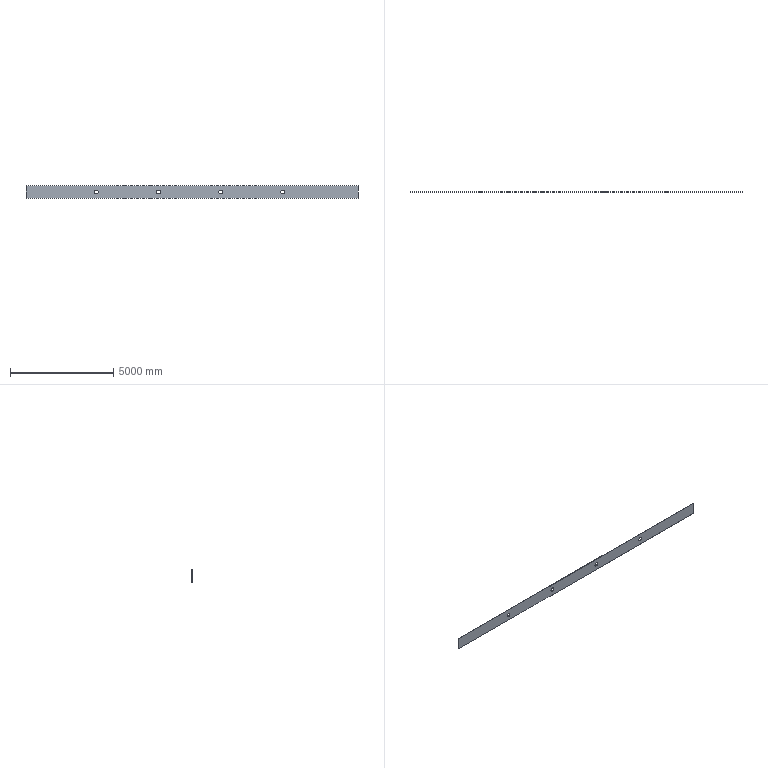Part | SolidWorks | features Cut 1, Extrusion 1, LPattern 1 | 1 solid | 14 faces | box 16040 x 12 x 600 mm | volume 114266549 mm3 | cylinder 8 | plane 6 | commonest cylinder face diameters 180 x8
STEP:
#1=CARTESIAN_POINT('',(-1620.,0.,-90.));
#2=VERTEX_POINT('',#1);
#3=CARTESIAN_POINT('',(-1620.,0.,90.));
#4=VERTEX_POINT('',#3);
#5=CARTESIAN_POINT('',(-1620.,0.,0.));
#6=DIRECTION('',(0.,1.,0.));
#7=DIRECTION('',(0.,0.,1.));
#8=AXIS2_PLACEMENT_3D('',#5,#6,#7);
#9=CIRCLE('',#8,90.);
#10=EDGE_CURVE('',#2,#4,#9,.T.);
#11=ORIENTED_EDGE('',*,*,#10,.F.);
#12=CARTESIAN_POINT('',(-1620.,12.,-90.));
#13=VERTEX_POINT('',#12);
#14=CARTESIAN_POINT('',(-1620.,0.,-90.));
#15=DIRECTION('',(0.,1.,0.));
#16=VECTOR('',#15,1000.);
#17=LINE('',#14,#16);
#18=EDGE_CURVE('',#2,#13,#17,.T.);
#19=ORIENTED_EDGE('',*,*,#18,.T.);
#20=CARTESIAN_POINT('',(-1620.,12.,90.));
#21=VERTEX_POINT('',#20);
#22=CARTESIAN_POINT('',(-1620.,12.,0.));
#23=DIRECTION('',(0.,1.,0.));
#24=DIRECTION('',(0.,0.,1.));
#25=AXIS2_PLACEMENT_3D('',#22,#23,#24);
#26=CIRCLE('',#25,90.);
#27=EDGE_CURVE('',#13,#21,#26,.T.);
#28=ORIENTED_EDGE('',*,*,#27,.T.);
#29=CARTESIAN_POINT('',(-1620.,0.,90.));
#30=DIRECTION('',(0.,1.,0.));
#31=VECTOR('',#30,1000.);
#32=LINE('',#29,#31);
#33=EDGE_CURVE('',#4,#21,#32,.T.);
#34=ORIENTED_EDGE('',*,*,#33,.F.);
#35=EDGE_LOOP('',(#11,#19,#28,#34));
#36=FACE_OUTER_BOUND('',#35,.T.);
#37=CARTESIAN_POINT('',(-1620.,0.,0.));
#38=DIRECTION('',(0.,1.,0.));
#39=DIRECTION('',(0.,0.,1.));
#40=AXIS2_PLACEMENT_3D('',#37,#38,#39);
#41=CYLINDRICAL_SURFACE('',#40,90.);
#42=ADVANCED_FACE('',(#36),#41,.F.);
#43=CARTESIAN_POINT('',(-4620.,0.,-90.));
#44=VERTEX_POINT('',#43);
#45=CARTESIAN_POINT('',(-4620.,0.,90.));
#46=VERTEX_POINT('',#45);
#47=CARTESIAN_POINT('',(-4620.,0.,0.));
#48=DIRECTION('',(0.,1.,0.));
#49=DIRECTION('',(0.,0.,1.));
#50=AXIS2_PLACEMENT_3D('',#47,#48,#49);
#51=CIRCLE('',#50,90.);
#52=EDGE_CURVE('',#44,#46,#51,.T.);
#53=ORIENTED_EDGE('',*,*,#52,.F.);
#54=CARTESIAN_POINT('',(-4620.,12.,-90.));
#55=VERTEX_POINT('',#54);
#56=CARTESIAN_POINT('',(-4620.,0.,-90.));
#57=DIRECTION('',(0.,1.,0.));
#58=VECTOR('',#57,1000.);
#59=LINE('',#56,#58);
#60=EDGE_CURVE('',#44,#55,#59,.T.);
#61=ORIENTED_EDGE('',*,*,#60,.T.);
#62=CARTESIAN_POINT('',(-4620.,12.,90.));
#63=VERTEX_POINT('',#62);
#64=CARTESIAN_POINT('',(-4620.,12.,0.));
#65=DIRECTION('',(0.,1.,0.));
#66=DIRECTION('',(0.,0.,1.));
#67=AXIS2_PLACEMENT_3D('',#64,#65,#66);
#68=CIRCLE('',#67,90.);
#69=EDGE_CURVE('',#55,#63,#68,.T.);
#70=ORIENTED_EDGE('',*,*,#69,.T.);
#71=CARTESIAN_POINT('',(-4620.,0.,90.));
#72=DIRECTION('',(0.,1.,0.));
#73=VECTOR('',#72,1000.);
#74=LINE('',#71,#73);
#75=EDGE_CURVE('',#46,#63,#74,.T.);
#76=ORIENTED_EDGE('',*,*,#75,.F.);
#77=EDGE_LOOP('',(#53,#61,#70,#76));
#78=FACE_OUTER_BOUND('',#77,.T.);
#79=CARTESIAN_POINT('',(-4620.,0.,0.));
#80=DIRECTION('',(0.,1.,0.));
#81=DIRECTION('',(0.,0.,1.));
#82=AXIS2_PLACEMENT_3D('',#79,#80,#81);
#83=CYLINDRICAL_SURFACE('',#82,90.);
#84=ADVANCED_FACE('',(#78),#83,.F.);
#85=CARTESIAN_POINT('',(1380.,0.,-90.));
#86=VERTEX_POINT('',#85);
#87=CARTESIAN_POINT('',(1380.,0.,90.));
#88=VERTEX_POINT('',#87);
#89=CARTESIAN_POINT('',(1380.,0.,0.));
#90=DIRECTION('',(0.,1.,0.));
#91=DIRECTION('',(0.,0.,1.));
#92=AXIS2_PLACEMENT_3D('',#89,#90,#91);
#93=CIRCLE('',#92,90.);
#94=EDGE_CURVE('',#86,#88,#93,.T.);
#95=ORIENTED_EDGE('',*,*,#94,.F.);
#96=CARTESIAN_POINT('',(1380.,12.,-90.));
#97=VERTEX_POINT('',#96);
#98=CARTESIAN_POINT('',(1380.,0.,-90.));
#99=DIRECTION('',(0.,1.,0.));
#100=VECTOR('',#99,1000.);
#101=LINE('',#98,#100);
#102=EDGE_CURVE('',#86,#97,#101,.T.);
#103=ORIENTED_EDGE('',*,*,#102,.T.);
#104=CARTESIAN_POINT('',(1380.,12.,90.));
#105=VERTEX_POINT('',#104);
#106=CARTESIAN_POINT('',(1380.,12.,0.));
#107=DIRECTION('',(0.,1.,0.));
#108=DIRECTION('',(0.,0.,1.));
#109=AXIS2_PLACEMENT_3D('',#106,#107,#108);
#110=CIRCLE('',#109,90.);
#111=EDGE_CURVE('',#97,#105,#110,.T.);
#112=ORIENTED_EDGE('',*,*,#111,.T.);
#113=CARTESIAN_POINT('',(1380.,0.,90.));
#114=DIRECTION('',(0.,1.,0.));
#115=VECTOR('',#114,1000.);
#116=LINE('',#113,#115);
#117=EDGE_CURVE('',#88,#105,#116,.T.);
#118=ORIENTED_EDGE('',*,*,#117,.F.);
#119=EDGE_LOOP('',(#95,#103,#112,#118));
#120=FACE_OUTER_BOUND('',#119,.T.);
#121=CARTESIAN_POINT('',(1380.,0.,0.));
#122=DIRECTION('',(0.,1.,0.));
#123=DIRECTION('',(0.,0.,1.));
#124=AXIS2_PLACEMENT_3D('',#121,#122,#123);
#125=CYLINDRICAL_SURFACE('',#124,90.);
#126=ADVANCED_FACE('',(#120),#125,.F.);
#127=CARTESIAN_POINT('',(4380.,0.,-90.));
#128=VERTEX_POINT('',#127);
#129=CARTESIAN_POINT('',(4380.,0.,90.));
#130=VERTEX_POINT('',#129);
#131=CARTESIAN_POINT('',(4380.,0.,0.));
#132=DIRECTION('',(0.,1.,0.));
#133=DIRECTION('',(0.,0.,1.));
#134=AXIS2_PLACEMENT_3D('',#131,#132,#133);
#135=CIRCLE('',#134,90.);
#136=EDGE_CURVE('',#128,#130,#135,.T.);
#137=ORIENTED_EDGE('',*,*,#136,.F.);
#138=CARTESIAN_POINT('',(4380.,12.,-90.));
#139=VERTEX_POINT('',#138);
#140=CARTESIAN_POINT('',(4380.,0.,-90.));
#141=DIRECTION('',(0.,1.,0.));
#142=VECTOR('',#141,1000.);
#143=LINE('',#140,#142);
#144=EDGE_CURVE('',#128,#139,#143,.T.);
#145=ORIENTED_EDGE('',*,*,#144,.T.);
#146=CARTESIAN_POINT('',(4380.,12.,90.));
#147=VERTEX_POINT('',#146);
#148=CARTESIAN_POINT('',(4380.,12.,0.));
#149=DIRECTION('',(0.,1.,0.));
#150=DIRECTION('',(0.,0.,1.));
#151=AXIS2_PLACEMENT_3D('',#148,#149,#150);
#152=CIRCLE('',#151,90.);
#153=EDGE_CURVE('',#139,#147,#152,.T.);
#154=ORIENTED_EDGE('',*,*,#153,.T.);
#155=CARTESIAN_POINT('',(4380.,0.,90.));
#156=DIRECTION('',(0.,1.,0.));
#157=VECTOR('',#156,1000.);
#158=LINE('',#155,#157);
#159=EDGE_CURVE('',#130,#147,#158,.T.);
#160=ORIENTED_EDGE('',*,*,#159,.F.);
#161=EDGE_LOOP('',(#137,#145,#154,#160));
#162=FACE_OUTER_BOUND('',#161,.T.);
#163=CARTESIAN_POINT('',(4380.,0.,0.));
#164=DIRECTION('',(0.,1.,0.));
#165=DIRECTION('',(0.,0.,1.));
#166=AXIS2_PLACEMENT_3D('',#163,#164,#165);
#167=CYLINDRICAL_SURFACE('',#166,90.);
#168=ADVANCED_FACE('',(#162),#167,.F.);
#169=ORIENTED_EDGE('',*,*,#144,.F.);
#170=CARTESIAN_POINT('',(4380.,0.,0.));
#171=DIRECTION('',(0.,1.,0.));
#172=DIRECTION('',(0.,0.,1.));
#173=AXIS2_PLACEMENT_3D('',#170,#171,#172);
#174=CIRCLE('',#173,90.);
#175=EDGE_CURVE('',#130,#128,#174,.T.);
#176=ORIENTED_EDGE('',*,*,#175,.F.);
#177=ORIENTED_EDGE('',*,*,#159,.T.);
#178=CARTESIAN_POINT('',(4380.,12.,0.));
#179=DIRECTION('',(0.,1.,0.));
#180=DIRECTION('',(0.,0.,1.));
#181=AXIS2_PLACEMENT_3D('',#178,#179,#180);
#182=CIRCLE('',#181,90.);
#183=EDGE_CURVE('',#147,#139,#182,.T.);
#184=ORIENTED_EDGE('',*,*,#183,.T.);
#185=EDGE_LOOP('',(#169,#176,#177,#184));
#186=FACE_OUTER_BOUND('',#185,.T.);
#187=CARTESIAN_POINT('',(4380.,0.,0.));
#188=DIRECTION('',(0.,1.,0.));
#189=DIRECTION('',(0.,0.,1.));
#190=AXIS2_PLACEMENT_3D('',#187,#188,#189);
#191=CYLINDRICAL_SURFACE('',#190,90.);
#192=ADVANCED_FACE('',(#186),#191,.F.);
#193=ORIENTED_EDGE('',*,*,#102,.F.);
#194=CARTESIAN_POINT('',(1380.,0.,0.));
#195=DIRECTION('',(0.,1.,0.));
#196=DIRECTION('',(0.,0.,1.));
#197=AXIS2_PLACEMENT_3D('',#194,#195,#196);
#198=CIRCLE('',#197,90.);
#199=EDGE_CURVE('',#88,#86,#198,.T.);
#200=ORIENTED_EDGE('',*,*,#199,.F.);
#201=ORIENTED_EDGE('',*,*,#117,.T.);
#202=CARTESIAN_POINT('',(1380.,12.,0.));
#203=DIRECTION('',(0.,1.,0.));
#204=DIRECTION('',(0.,0.,1.));
#205=AXIS2_PLACEMENT_3D('',#202,#203,#204);
#206=CIRCLE('',#205,90.);
#207=EDGE_CURVE('',#105,#97,#206,.T.);
#208=ORIENTED_EDGE('',*,*,#207,.T.);
#209=EDGE_LOOP('',(#193,#200,#201,#208));
#210=FACE_OUTER_BOUND('',#209,.T.);
#211=CARTESIAN_POINT('',(1380.,0.,0.));
#212=DIRECTION('',(0.,1.,0.));
#213=DIRECTION('',(0.,0.,1.));
#214=AXIS2_PLACEMENT_3D('',#211,#212,#213);
#215=CYLINDRICAL_SURFACE('',#214,90.);
#216=ADVANCED_FACE('',(#210),#215,.F.);
#217=CARTESIAN_POINT('',(8020.,0.,300.));
#218=VERTEX_POINT('',#217);
#219=CARTESIAN_POINT('',(8020.,0.,-300.));
#220=VERTEX_POINT('',#219);
#221=CARTESIAN_POINT('',(8020.,0.,-300.));
#222=DIRECTION('',(0.,0.,-1.));
#223=VECTOR('',#222,1000.);
#224=LINE('',#221,#223);
#225=EDGE_CURVE('',#218,#220,#224,.T.);
#226=ORIENTED_EDGE('',*,*,#225,.T.);
#227=CARTESIAN_POINT('',(8020.,12.,-300.));
#228=VERTEX_POINT('',#227);
#229=CARTESIAN_POINT('',(8020.,12.,-300.));
#230=DIRECTION('',(0.,-1.,0.));
#231=VECTOR('',#230,1000.);
#232=LINE('',#229,#231);
#233=EDGE_CURVE('',#228,#220,#232,.T.);
#234=ORIENTED_EDGE('',*,*,#233,.F.);
#235=CARTESIAN_POINT('',(8020.,12.,300.));
#236=VERTEX_POINT('',#235);
#237=CARTESIAN_POINT('',(8020.,12.,-300.));
#238=DIRECTION('',(0.,0.,-1.));
#239=VECTOR('',#238,1000.);
#240=LINE('',#237,#239);
#241=EDGE_CURVE('',#236,#228,#240,.T.);
#242=ORIENTED_EDGE('',*,*,#241,.F.);
#243=CARTESIAN_POINT('',(8020.,12.,300.));
#244=DIRECTION('',(0.,-1.,0.));
#245=VECTOR('',#244,1000.);
#246=LINE('',#243,#245);
#247=EDGE_CURVE('',#236,#218,#246,.T.);
#248=ORIENTED_EDGE('',*,*,#247,.T.);
#249=EDGE_LOOP('',(#226,#234,#242,#248));
#250=FACE_OUTER_BOUND('',#249,.T.);
#251=CARTESIAN_POINT('',(8020.,12.,-300.));
#252=DIRECTION('',(-1.,0.,0.));
#253=DIRECTION('',(0.,0.,1.));
#254=AXIS2_PLACEMENT_3D('',#251,#252,#253);
#255=PLANE('',#254);
#256=ADVANCED_FACE('',(#250),#255,.F.);
#257=CARTESIAN_POINT('',(-8020.,0.,-300.));
#258=VERTEX_POINT('',#257);
#259=CARTESIAN_POINT('',(-8020.,0.,-300.));
#260=DIRECTION('',(-1.,0.,0.));
#261=VECTOR('',#260,1000.);
#262=LINE('',#259,#261);
#263=EDGE_CURVE('',#220,#258,#262,.T.);
#264=ORIENTED_EDGE('',*,*,#263,.T.);
#265=CARTESIAN_POINT('',(-8020.,12.,-300.));
#266=VERTEX_POINT('',#265);
#267=CARTESIAN_POINT('',(-8020.,12.,-300.));
#268=DIRECTION('',(0.,-1.,0.));
#269=VECTOR('',#268,1000.);
#270=LINE('',#267,#269);
#271=EDGE_CURVE('',#266,#258,#270,.T.);
#272=ORIENTED_EDGE('',*,*,#271,.F.);
#273=CARTESIAN_POINT('',(-8020.,12.,-300.));
#274=DIRECTION('',(-1.,0.,0.));
#275=VECTOR('',#274,1000.);
#276=LINE('',#273,#275);
#277=EDGE_CURVE('',#228,#266,#276,.T.);
#278=ORIENTED_EDGE('',*,*,#277,.F.);
#279=ORIENTED_EDGE('',*,*,#233,.T.);
#280=EDGE_LOOP('',(#264,#272,#278,#279));
#281=FACE_OUTER_BOUND('',#280,.T.);
#282=CARTESIAN_POINT('',(-8020.,12.,-300.));
#283=DIRECTION('',(0.,0.,1.));
#284=DIRECTION('',(1.,0.,0.));
#285=AXIS2_PLACEMENT_3D('',#282,#283,#284);
#286=PLANE('',#285);
#287=ADVANCED_FACE('',(#281),#286,.F.);
#288=CARTESIAN_POINT('',(-8020.,0.,300.));
#289=VERTEX_POINT('',#288);
#290=CARTESIAN_POINT('',(-8020.,0.,-300.));
#291=DIRECTION('',(0.,0.,1.));
#292=VECTOR('',#291,1000.);
#293=LINE('',#290,#292);
#294=EDGE_CURVE('',#258,#289,#293,.T.);
#295=ORIENTED_EDGE('',*,*,#294,.T.);
#296=CARTESIAN_POINT('',(-8020.,12.,300.));
#297=VERTEX_POINT('',#296);
#298=CARTESIAN_POINT('',(-8020.,12.,300.));
#299=DIRECTION('',(0.,-1.,0.));
#300=VECTOR('',#299,1000.);
#301=LINE('',#298,#300);
#302=EDGE_CURVE('',#297,#289,#301,.T.);
#303=ORIENTED_EDGE('',*,*,#302,.F.);
#304=CARTESIAN_POINT('',(-8020.,12.,-300.));
#305=DIRECTION('',(0.,0.,1.));
#306=VECTOR('',#305,1000.);
#307=LINE('',#304,#306);
#308=EDGE_CURVE('',#266,#297,#307,.T.);
#309=ORIENTED_EDGE('',*,*,#308,.F.);
#310=ORIENTED_EDGE('',*,*,#271,.T.);
#311=EDGE_LOOP('',(#295,#303,#309,#310));
#312=FACE_OUTER_BOUND('',#311,.T.);
#313=CARTESIAN_POINT('',(-8020.,12.,-300.));
#314=DIRECTION('',(1.,0.,0.));
#315=DIRECTION('',(0.,0.,-1.));
#316=AXIS2_PLACEMENT_3D('',#313,#314,#315);
#317=PLANE('',#316);
#318=ADVANCED_FACE('',(#312),#317,.F.);
#319=CARTESIAN_POINT('',(-8020.,0.,300.));
#320=DIRECTION('',(1.,0.,0.));
#321=VECTOR('',#320,1000.);
#322=LINE('',#319,#321);
#323=EDGE_CURVE('',#289,#218,#322,.T.);
#324=ORIENTED_EDGE('',*,*,#323,.T.);
#325=ORIENTED_EDGE('',*,*,#247,.F.);
#326=CARTESIAN_POINT('',(-8020.,12.,300.));
#327=DIRECTION('',(1.,0.,0.));
#328=VECTOR('',#327,1000.);
#329=LINE('',#326,#328);
#330=EDGE_CURVE('',#297,#236,#329,.T.);
#331=ORIENTED_EDGE('',*,*,#330,.F.);
#332=ORIENTED_EDGE('',*,*,#302,.T.);
#333=EDGE_LOOP('',(#324,#325,#331,#332));
#334=FACE_OUTER_BOUND('',#333,.T.);
#335=CARTESIAN_POINT('',(-8020.,12.,300.));
#336=DIRECTION('',(0.,0.,-1.));
#337=DIRECTION('',(-1.,0.,0.));
#338=AXIS2_PLACEMENT_3D('',#335,#336,#337);
#339=PLANE('',#338);
#340=ADVANCED_FACE('',(#334),#339,.F.);
#341=CARTESIAN_POINT('',(-1620.,12.,0.));
#342=DIRECTION('',(0.,1.,0.));
#343=DIRECTION('',(0.,0.,1.));
#344=AXIS2_PLACEMENT_3D('',#341,#342,#343);
#345=CIRCLE('',#344,90.);
#346=EDGE_CURVE('',#21,#13,#345,.T.);
#347=ORIENTED_EDGE('',*,*,#346,.F.);
#348=ORIENTED_EDGE('',*,*,#27,.F.);
#349=EDGE_LOOP('',(#347,#348));
#350=FACE_BOUND('',#349,.T.);
#351=CARTESIAN_POINT('',(-4620.,12.,0.));
#352=DIRECTION('',(0.,1.,0.));
#353=DIRECTION('',(0.,0.,1.));
#354=AXIS2_PLACEMENT_3D('',#351,#352,#353);
#355=CIRCLE('',#354,90.);
#356=EDGE_CURVE('',#63,#55,#355,.T.);
#357=ORIENTED_EDGE('',*,*,#356,.F.);
#358=ORIENTED_EDGE('',*,*,#69,.F.);
#359=EDGE_LOOP('',(#357,#358));
#360=FACE_BOUND('',#359,.T.);
#361=ORIENTED_EDGE('',*,*,#241,.T.);
#362=ORIENTED_EDGE('',*,*,#277,.T.);
#363=ORIENTED_EDGE('',*,*,#308,.T.);
#364=ORIENTED_EDGE('',*,*,#330,.T.);
#365=EDGE_LOOP('',(#361,#362,#363,#364));
#366=FACE_OUTER_BOUND('',#365,.T.);
#367=ORIENTED_EDGE('',*,*,#207,.F.);
#368=ORIENTED_EDGE('',*,*,#111,.F.);
#369=EDGE_LOOP('',(#367,#368));
#370=FACE_BOUND('',#369,.T.);
#371=ORIENTED_EDGE('',*,*,#183,.F.);
#372=ORIENTED_EDGE('',*,*,#153,.F.);
#373=EDGE_LOOP('',(#371,#372));
#374=FACE_BOUND('',#373,.T.);
#375=CARTESIAN_POINT('',(0.,12.,0.));
#376=DIRECTION('',(0.,1.,0.));
#377=DIRECTION('',(0.,0.,1.));
#378=AXIS2_PLACEMENT_3D('',#375,#376,#377);
#379=PLANE('',#378);
#380=ADVANCED_FACE('',(#350,#360,#366,#370,#374),#379,.T.);
#381=CARTESIAN_POINT('',(-1620.,0.,0.));
#382=DIRECTION('',(0.,1.,0.));
#383=DIRECTION('',(0.,0.,1.));
#384=AXIS2_PLACEMENT_3D('',#381,#382,#383);
#385=CIRCLE('',#384,90.);
#386=EDGE_CURVE('',#4,#2,#385,.T.);
#387=ORIENTED_EDGE('',*,*,#386,.T.);
#388=ORIENTED_EDGE('',*,*,#10,.T.);
#389=EDGE_LOOP('',(#387,#388));
#390=FACE_BOUND('',#389,.T.);
#391=CARTESIAN_POINT('',(-4620.,0.,0.));
#392=DIRECTION('',(0.,1.,0.));
#393=DIRECTION('',(0.,0.,1.));
#394=AXIS2_PLACEMENT_3D('',#391,#392,#393);
#395=CIRCLE('',#394,90.);
#396=EDGE_CURVE('',#46,#44,#395,.T.);
#397=ORIENTED_EDGE('',*,*,#396,.T.);
#398=ORIENTED_EDGE('',*,*,#52,.T.);
#399=EDGE_LOOP('',(#397,#398));
#400=FACE_BOUND('',#399,.T.);
#401=ORIENTED_EDGE('',*,*,#225,.F.);
#402=ORIENTED_EDGE('',*,*,#323,.F.);
#403=ORIENTED_EDGE('',*,*,#294,.F.);
#404=ORIENTED_EDGE('',*,*,#263,.F.);
#405=EDGE_LOOP('',(#401,#402,#403,#404));
#406=FACE_OUTER_BOUND('',#405,.T.);
#407=ORIENTED_EDGE('',*,*,#199,.T.);
#408=ORIENTED_EDGE('',*,*,#94,.T.);
#409=EDGE_LOOP('',(#407,#408));
#410=FACE_BOUND('',#409,.T.);
#411=ORIENTED_EDGE('',*,*,#175,.T.);
#412=ORIENTED_EDGE('',*,*,#136,.T.);
#413=EDGE_LOOP('',(#411,#412));
#414=FACE_BOUND('',#413,.T.);
#415=CARTESIAN_POINT('',(0.,0.,0.));
#416=DIRECTION('',(0.,1.,0.));
#417=DIRECTION('',(0.,0.,1.));
#418=AXIS2_PLACEMENT_3D('',#415,#416,#417);
#419=PLANE('',#418);
#420=ADVANCED_FACE('',(#390,#400,#406,#410,#414),#419,.F.);
#421=ORIENTED_EDGE('',*,*,#60,.F.);
#422=ORIENTED_EDGE('',*,*,#396,.F.);
#423=ORIENTED_EDGE('',*,*,#75,.T.);
#424=ORIENTED_EDGE('',*,*,#356,.T.);
#425=EDGE_LOOP('',(#421,#422,#423,#424));
#426=FACE_OUTER_BOUND('',#425,.T.);
#427=CARTESIAN_POINT('',(-4620.,0.,0.));
#428=DIRECTION('',(0.,1.,0.));
#429=DIRECTION('',(0.,0.,1.));
#430=AXIS2_PLACEMENT_3D('',#427,#428,#429);
#431=CYLINDRICAL_SURFACE('',#430,90.);
#432=ADVANCED_FACE('',(#426),#431,.F.);
#433=ORIENTED_EDGE('',*,*,#18,.F.);
#434=ORIENTED_EDGE('',*,*,#386,.F.);
#435=ORIENTED_EDGE('',*,*,#33,.T.);
#436=ORIENTED_EDGE('',*,*,#346,.T.);
#437=EDGE_LOOP('',(#433,#434,#435,#436));
#438=FACE_OUTER_BOUND('',#437,.T.);
#439=CARTESIAN_POINT('',(-1620.,0.,0.));
#440=DIRECTION('',(0.,1.,0.));
#441=DIRECTION('',(0.,0.,1.));
#442=AXIS2_PLACEMENT_3D('',#439,#440,#441);
#443=CYLINDRICAL_SURFACE('',#442,90.);
#444=ADVANCED_FACE('',(#438),#443,.F.);
#445=CLOSED_SHELL('',(#42,#84,#126,#168,#192,#216,#256,#287,#318,#340,#380,#420,#432,#444));
#446=MANIFOLD_SOLID_BREP('',#445);
#447=CARTESIAN_POINT('',(0.,0.,0.));
#448=DIRECTION('',(0.,0.,1.));
#449=DIRECTION('',(1.,0.,0.));
#450=AXIS2_PLACEMENT_3D('',#447,#448,#449);
#451=(LENGTH_UNIT()NAMED_UNIT(*)SI_UNIT(.MILLI.,.METRE.));
#452=UNCERTAINTY_MEASURE_WITH_UNIT(LENGTH_MEASURE(0.00001),#451,'','');
#453=(NAMED_UNIT(*)PLANE_ANGLE_UNIT()SI_UNIT($,.RADIAN.));
#454=(NAMED_UNIT(*)SI_UNIT($,.STERADIAN.)SOLID_ANGLE_UNIT());
#455=(GEOMETRIC_REPRESENTATION_CONTEXT(3)GLOBAL_UNCERTAINTY_ASSIGNED_CONTEXT((#452))GLOBAL_UNIT_ASSIGNED_CONTEXT((#451,#453,#454))REPRESENTATION_CONTEXT('',''));
#456=ADVANCED_BREP_SHAPE_REPRESENTATION('',(#446,#450),#455);